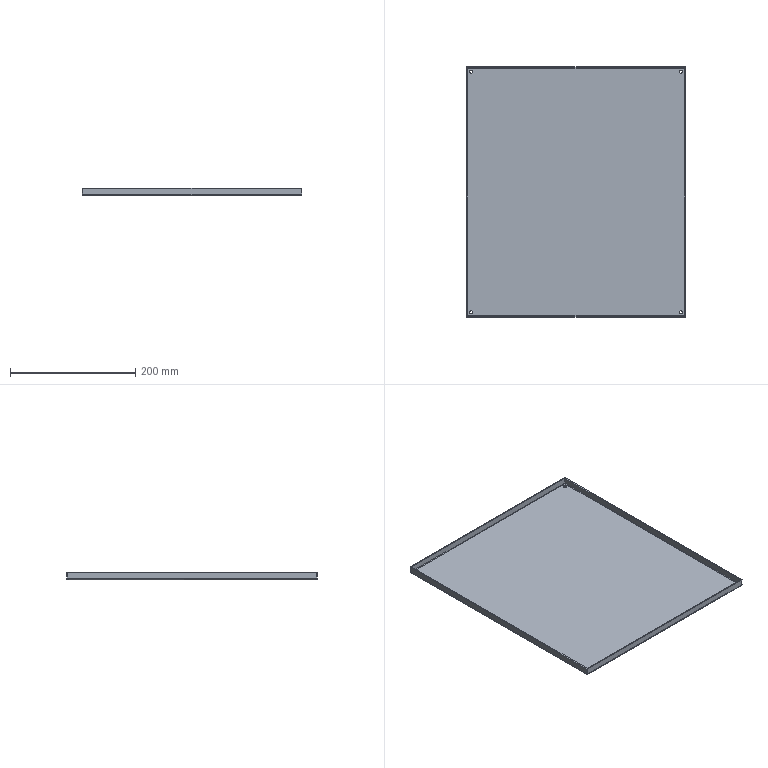Part | STEP file | Lower control board 11 | 1 solid | 51 faces | box 350 x 400 x 12 mm | volume 307444 mm3 | cylinder 20 | spline 20 | plane 11 | commonest cylinder face diameters 5 x8 1.473 x4 2 x4 5.473 x4